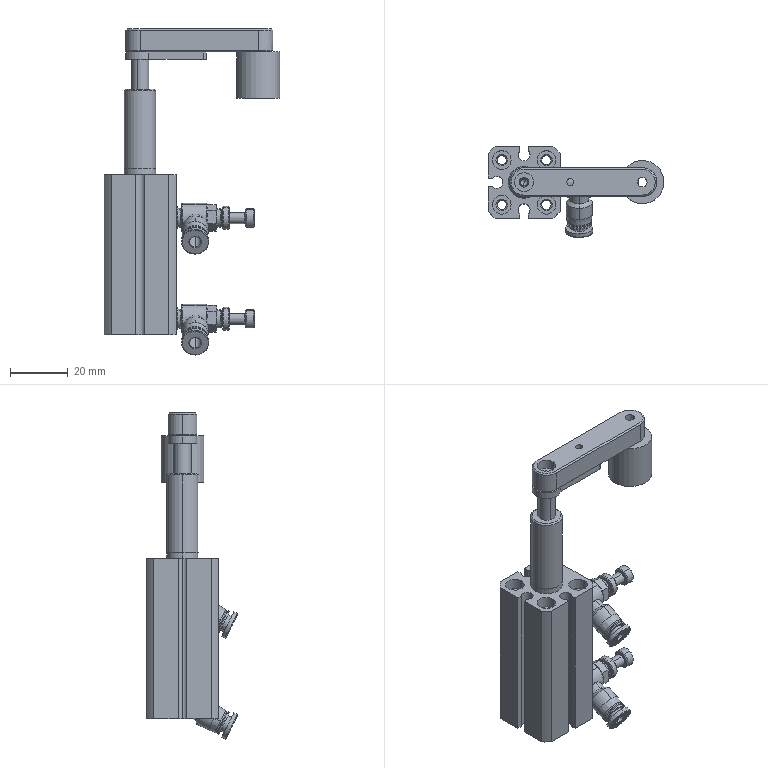Part | SolidWorks | 7 solids | 466 faces | box 61 x 31.574 x 113.094 mm | volume 38562 mm3 | cylinder 179 | plane 165 | cone 104 | spline 18 | commonest cylinder face diameters 6.5 x22 3.242 x16 4 x12 10 x9 3.5 x8 4.15 x8